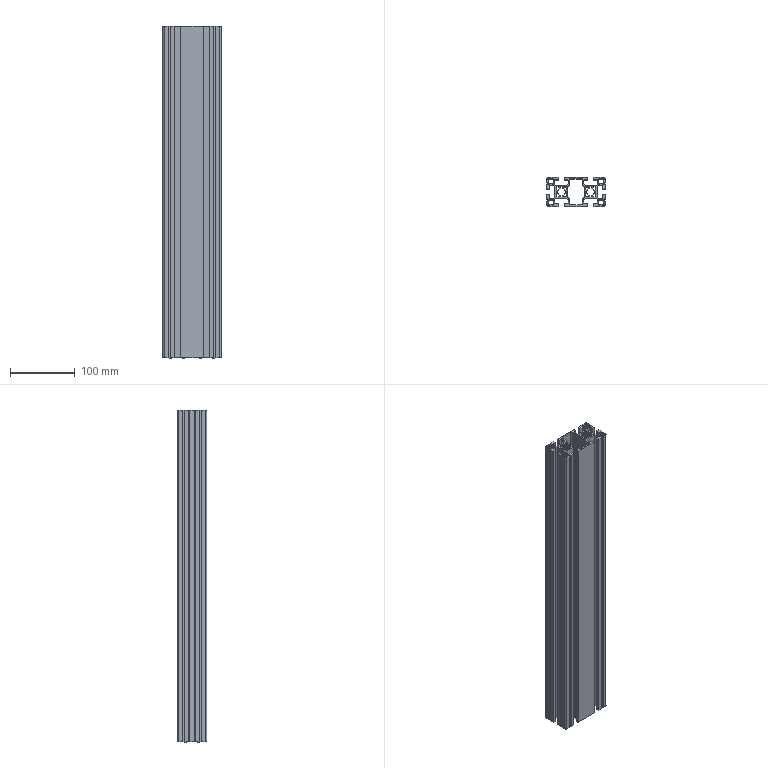Part | STEP file | 4590-615 aluminium profile (rear middle upright 2) | 1 solid | 366 faces | box 90 x 45 x 513 mm | volume 601597 mm3 | plane 254 | cylinder 112 | commonest cylinder face diameters 2 x64 8 x20 12 x16 4 x12